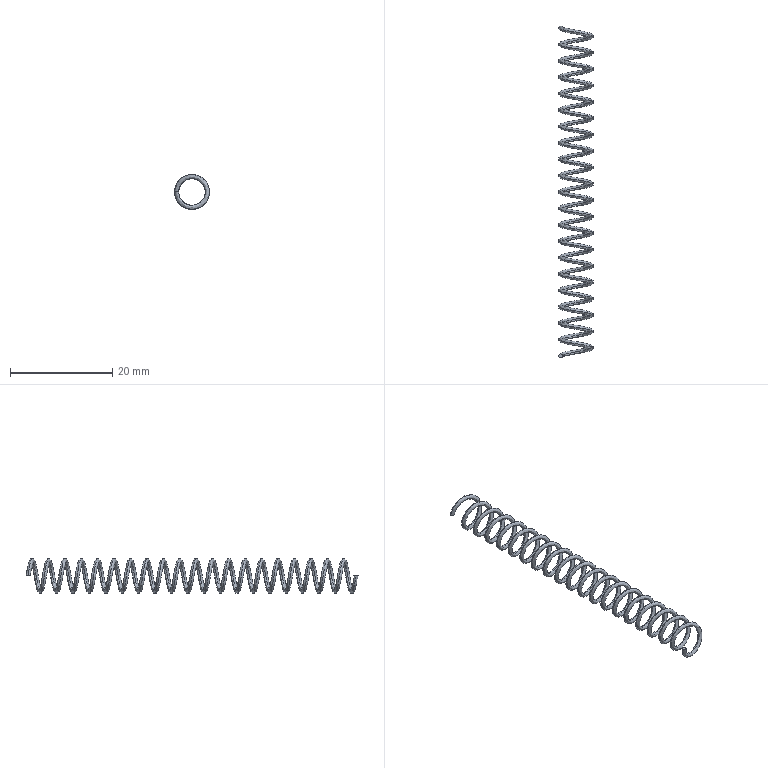Part | SolidWorks | features Sweep 1 | 1 solid | 4 faces | box 6.8 x 64.8 x 6.8 mm | volume 188.36 mm3 | spline 2 | plane 2